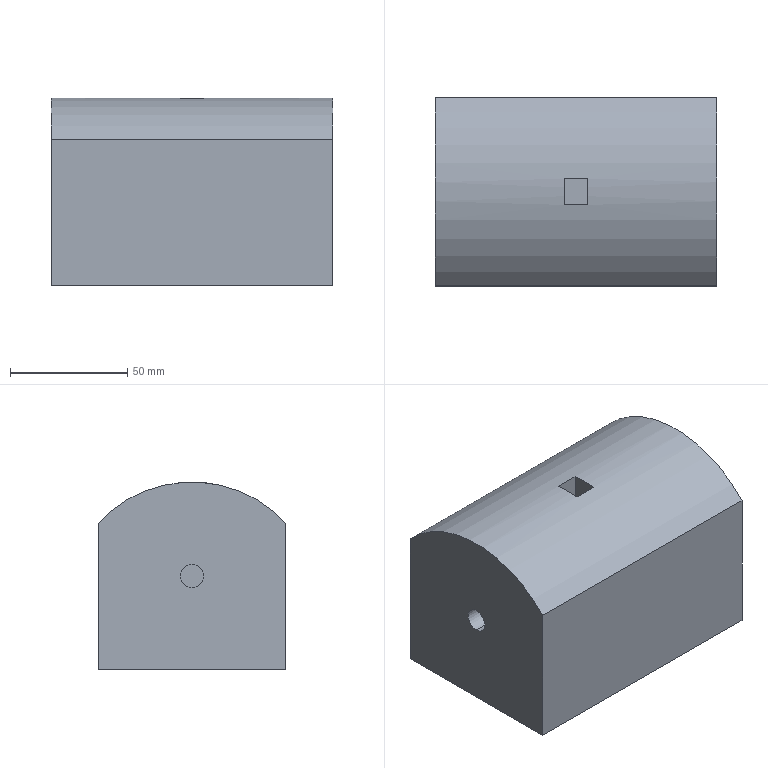Part | SolidWorks | features ICE 4, Extrusion 1 | 1 solid | 17 faces | box 120 x 80 x 80 mm | volume 704237 mm3 | plane 12 | cylinder 5 | commonest cylinder face diameters 10 x4 109 x1
STEP:
#1=CARTESIAN_POINT('',(60.,0.,35.));
#2=VERTEX_POINT('',#1);
#3=CARTESIAN_POINT('',(60.,0.,45.));
#4=VERTEX_POINT('',#3);
#5=CARTESIAN_POINT('',(60.,0.,40.));
#6=DIRECTION('',(-1.,0.,0.));
#7=DIRECTION('',(0.,0.,1.));
#8=AXIS2_PLACEMENT_3D('',#5,#6,#7);
#9=CIRCLE('',#8,5.);
#10=EDGE_CURVE('',#2,#4,#9,.T.);
#11=ORIENTED_EDGE('',*,*,#10,.F.);
#12=CARTESIAN_POINT('',(5.,0.,35.));
#13=VERTEX_POINT('',#12);
#14=CARTESIAN_POINT('',(60.,0.,35.));
#15=DIRECTION('',(-1.,0.,0.));
#16=VECTOR('',#15,1000.);
#17=LINE('',#14,#16);
#18=EDGE_CURVE('',#2,#13,#17,.T.);
#19=ORIENTED_EDGE('',*,*,#18,.T.);
#20=CARTESIAN_POINT('',(5.,0.,45.));
#21=VERTEX_POINT('',#20);
#22=CARTESIAN_POINT('',(5.,0.,40.));
#23=DIRECTION('',(1.,0.,0.));
#24=DIRECTION('',(0.,0.,-1.));
#25=AXIS2_PLACEMENT_3D('',#22,#23,#24);
#26=CIRCLE('',#25,5.);
#27=EDGE_CURVE('',#21,#13,#26,.T.);
#28=ORIENTED_EDGE('',*,*,#27,.F.);
#29=CARTESIAN_POINT('',(60.,0.,45.));
#30=DIRECTION('',(-1.,0.,0.));
#31=VECTOR('',#30,1000.);
#32=LINE('',#29,#31);
#33=EDGE_CURVE('',#4,#21,#32,.T.);
#34=ORIENTED_EDGE('',*,*,#33,.F.);
#35=EDGE_LOOP('',(#11,#19,#28,#34));
#36=FACE_OUTER_BOUND('',#35,.T.);
#37=CARTESIAN_POINT('',(60.,0.,40.));
#38=DIRECTION('',(-1.,0.,0.));
#39=DIRECTION('',(0.,0.,1.));
#40=AXIS2_PLACEMENT_3D('',#37,#38,#39);
#41=CYLINDRICAL_SURFACE('',#40,5.);
#42=ADVANCED_FACE('',(#36),#41,.F.);
#43=CARTESIAN_POINT('',(-5.,0.,35.));
#44=VERTEX_POINT('',#43);
#45=CARTESIAN_POINT('',(-5.,0.,45.));
#46=VERTEX_POINT('',#45);
#47=CARTESIAN_POINT('',(-5.,0.,40.));
#48=DIRECTION('',(-1.,0.,0.));
#49=DIRECTION('',(0.,0.,1.));
#50=AXIS2_PLACEMENT_3D('',#47,#48,#49);
#51=CIRCLE('',#50,5.);
#52=EDGE_CURVE('',#44,#46,#51,.T.);
#53=ORIENTED_EDGE('',*,*,#52,.F.);
#54=CARTESIAN_POINT('',(-60.,0.,35.));
#55=VERTEX_POINT('',#54);
#56=CARTESIAN_POINT('',(60.,0.,35.));
#57=DIRECTION('',(-1.,0.,0.));
#58=VECTOR('',#57,1000.);
#59=LINE('',#56,#58);
#60=EDGE_CURVE('',#44,#55,#59,.T.);
#61=ORIENTED_EDGE('',*,*,#60,.T.);
#62=CARTESIAN_POINT('',(-60.,0.,45.));
#63=VERTEX_POINT('',#62);
#64=CARTESIAN_POINT('',(-60.,0.,40.));
#65=DIRECTION('',(-1.,0.,0.));
#66=DIRECTION('',(0.,0.,1.));
#67=AXIS2_PLACEMENT_3D('',#64,#65,#66);
#68=CIRCLE('',#67,5.);
#69=EDGE_CURVE('',#55,#63,#68,.T.);
#70=ORIENTED_EDGE('',*,*,#69,.T.);
#71=CARTESIAN_POINT('',(60.,0.,45.));
#72=DIRECTION('',(-1.,0.,0.));
#73=VECTOR('',#72,1000.);
#74=LINE('',#71,#73);
#75=EDGE_CURVE('',#46,#63,#74,.T.);
#76=ORIENTED_EDGE('',*,*,#75,.F.);
#77=EDGE_LOOP('',(#53,#61,#70,#76));
#78=FACE_OUTER_BOUND('',#77,.T.);
#79=CARTESIAN_POINT('',(60.,0.,40.));
#80=DIRECTION('',(-1.,0.,0.));
#81=DIRECTION('',(0.,0.,1.));
#82=AXIS2_PLACEMENT_3D('',#79,#80,#81);
#83=CYLINDRICAL_SURFACE('',#82,5.);
#84=ADVANCED_FACE('',(#78),#83,.F.);
#85=ORIENTED_EDGE('',*,*,#60,.F.);
#86=CARTESIAN_POINT('',(-5.,0.,40.));
#87=DIRECTION('',(-1.,0.,0.));
#88=DIRECTION('',(0.,0.,1.));
#89=AXIS2_PLACEMENT_3D('',#86,#87,#88);
#90=CIRCLE('',#89,5.);
#91=EDGE_CURVE('',#46,#44,#90,.T.);
#92=ORIENTED_EDGE('',*,*,#91,.F.);
#93=ORIENTED_EDGE('',*,*,#75,.T.);
#94=CARTESIAN_POINT('',(-60.,0.,40.));
#95=DIRECTION('',(-1.,0.,0.));
#96=DIRECTION('',(0.,0.,1.));
#97=AXIS2_PLACEMENT_3D('',#94,#95,#96);
#98=CIRCLE('',#97,5.);
#99=EDGE_CURVE('',#63,#55,#98,.T.);
#100=ORIENTED_EDGE('',*,*,#99,.T.);
#101=EDGE_LOOP('',(#85,#92,#93,#100));
#102=FACE_OUTER_BOUND('',#101,.T.);
#103=CARTESIAN_POINT('',(60.,0.,40.));
#104=DIRECTION('',(-1.,0.,0.));
#105=DIRECTION('',(0.,0.,1.));
#106=AXIS2_PLACEMENT_3D('',#103,#104,#105);
#107=CYLINDRICAL_SURFACE('',#106,5.);
#108=ADVANCED_FACE('',(#102),#107,.F.);
#109=CARTESIAN_POINT('',(60.,0.,40.));
#110=DIRECTION('',(-1.,0.,0.));
#111=DIRECTION('',(0.,0.,1.));
#112=AXIS2_PLACEMENT_3D('',#109,#110,#111);
#113=CIRCLE('',#112,5.);
#114=EDGE_CURVE('',#4,#2,#113,.T.);
#115=ORIENTED_EDGE('',*,*,#114,.T.);
#116=ORIENTED_EDGE('',*,*,#10,.T.);
#117=EDGE_LOOP('',(#115,#116));
#118=FACE_BOUND('',#117,.T.);
#119=CARTESIAN_POINT('',(60.,40.,62.517));
#120=VERTEX_POINT('',#119);
#121=CARTESIAN_POINT('',(60.,-40.,62.517));
#122=VERTEX_POINT('',#121);
#123=CARTESIAN_POINT('',(60.,0.,25.5));
#124=DIRECTION('',(1.,0.,0.));
#125=DIRECTION('',(0.,0.,-1.));
#126=AXIS2_PLACEMENT_3D('',#123,#124,#125);
#127=CIRCLE('',#126,54.5);
#128=EDGE_CURVE('',#120,#122,#127,.T.);
#129=ORIENTED_EDGE('',*,*,#128,.T.);
#130=CARTESIAN_POINT('',(60.,-40.,0.));
#131=VERTEX_POINT('',#130);
#132=CARTESIAN_POINT('',(60.,-40.,80.));
#133=DIRECTION('',(0.,0.,-1.));
#134=VECTOR('',#133,1000.);
#135=LINE('',#132,#134);
#136=EDGE_CURVE('',#122,#131,#135,.T.);
#137=ORIENTED_EDGE('',*,*,#136,.T.);
#138=CARTESIAN_POINT('',(60.,40.,0.));
#139=VERTEX_POINT('',#138);
#140=CARTESIAN_POINT('',(60.,-40.,0.));
#141=DIRECTION('',(0.,1.,0.));
#142=VECTOR('',#141,1000.);
#143=LINE('',#140,#142);
#144=EDGE_CURVE('',#131,#139,#143,.T.);
#145=ORIENTED_EDGE('',*,*,#144,.T.);
#146=CARTESIAN_POINT('',(60.,40.,80.));
#147=DIRECTION('',(0.,0.,-1.));
#148=VECTOR('',#147,1000.);
#149=LINE('',#146,#148);
#150=EDGE_CURVE('',#120,#139,#149,.T.);
#151=ORIENTED_EDGE('',*,*,#150,.F.);
#152=EDGE_LOOP('',(#129,#137,#145,#151));
#153=FACE_OUTER_BOUND('',#152,.T.);
#154=CARTESIAN_POINT('',(60.,-40.,80.));
#155=DIRECTION('',(-1.,0.,0.));
#156=DIRECTION('',(0.,0.,1.));
#157=AXIS2_PLACEMENT_3D('',#154,#155,#156);
#158=PLANE('',#157);
#159=ADVANCED_FACE('',(#118,#153),#158,.F.);
#160=ORIENTED_EDGE('',*,*,#99,.F.);
#161=ORIENTED_EDGE('',*,*,#69,.F.);
#162=EDGE_LOOP('',(#160,#161));
#163=FACE_BOUND('',#162,.T.);
#164=CARTESIAN_POINT('',(-60.,-40.,62.517));
#165=VERTEX_POINT('',#164);
#166=CARTESIAN_POINT('',(-60.,-40.,0.));
#167=VERTEX_POINT('',#166);
#168=CARTESIAN_POINT('',(-60.,-40.,80.));
#169=DIRECTION('',(0.,0.,-1.));
#170=VECTOR('',#169,1000.);
#171=LINE('',#168,#170);
#172=EDGE_CURVE('',#165,#167,#171,.T.);
#173=ORIENTED_EDGE('',*,*,#172,.F.);
#174=CARTESIAN_POINT('',(-60.,40.,62.517));
#175=VERTEX_POINT('',#174);
#176=CARTESIAN_POINT('',(-60.,0.,25.5));
#177=DIRECTION('',(1.,0.,0.));
#178=DIRECTION('',(0.,0.,-1.));
#179=AXIS2_PLACEMENT_3D('',#176,#177,#178);
#180=CIRCLE('',#179,54.5);
#181=EDGE_CURVE('',#175,#165,#180,.T.);
#182=ORIENTED_EDGE('',*,*,#181,.F.);
#183=CARTESIAN_POINT('',(-60.,40.,0.));
#184=VERTEX_POINT('',#183);
#185=CARTESIAN_POINT('',(-60.,40.,80.));
#186=DIRECTION('',(0.,0.,-1.));
#187=VECTOR('',#186,1000.);
#188=LINE('',#185,#187);
#189=EDGE_CURVE('',#175,#184,#188,.T.);
#190=ORIENTED_EDGE('',*,*,#189,.T.);
#191=CARTESIAN_POINT('',(-60.,-40.,0.));
#192=DIRECTION('',(0.,-1.,0.));
#193=VECTOR('',#192,1000.);
#194=LINE('',#191,#193);
#195=EDGE_CURVE('',#184,#167,#194,.T.);
#196=ORIENTED_EDGE('',*,*,#195,.T.);
#197=EDGE_LOOP('',(#173,#182,#190,#196));
#198=FACE_OUTER_BOUND('',#197,.T.);
#199=CARTESIAN_POINT('',(-60.,-40.,80.));
#200=DIRECTION('',(1.,0.,0.));
#201=DIRECTION('',(0.,0.,-1.));
#202=AXIS2_PLACEMENT_3D('',#199,#200,#201);
#203=PLANE('',#202);
#204=ADVANCED_FACE('',(#163,#198),#203,.F.);
#205=CARTESIAN_POINT('',(-60.,-40.,62.517));
#206=DIRECTION('',(1.,0.,0.));
#207=VECTOR('',#206,1000.);
#208=LINE('',#205,#207);
#209=EDGE_CURVE('',#165,#122,#208,.T.);
#210=ORIENTED_EDGE('',*,*,#209,.F.);
#211=ORIENTED_EDGE('',*,*,#172,.T.);
#212=CARTESIAN_POINT('',(-60.,-40.,0.));
#213=DIRECTION('',(1.,0.,0.));
#214=VECTOR('',#213,1000.);
#215=LINE('',#212,#214);
#216=EDGE_CURVE('',#167,#131,#215,.T.);
#217=ORIENTED_EDGE('',*,*,#216,.T.);
#218=ORIENTED_EDGE('',*,*,#136,.F.);
#219=EDGE_LOOP('',(#210,#211,#217,#218));
#220=FACE_OUTER_BOUND('',#219,.T.);
#221=CARTESIAN_POINT('',(-60.,-40.,80.));
#222=DIRECTION('',(0.,1.,0.));
#223=DIRECTION('',(0.,0.,1.));
#224=AXIS2_PLACEMENT_3D('',#221,#222,#223);
#225=PLANE('',#224);
#226=ADVANCED_FACE('',(#220),#225,.F.);
#227=CARTESIAN_POINT('',(-60.,40.,62.517));
#228=DIRECTION('',(1.,0.,0.));
#229=VECTOR('',#228,1000.);
#230=LINE('',#227,#229);
#231=EDGE_CURVE('',#175,#120,#230,.T.);
#232=ORIENTED_EDGE('',*,*,#231,.T.);
#233=ORIENTED_EDGE('',*,*,#150,.T.);
#234=CARTESIAN_POINT('',(-60.,40.,0.));
#235=DIRECTION('',(-1.,0.,0.));
#236=VECTOR('',#235,1000.);
#237=LINE('',#234,#236);
#238=EDGE_CURVE('',#139,#184,#237,.T.);
#239=ORIENTED_EDGE('',*,*,#238,.T.);
#240=ORIENTED_EDGE('',*,*,#189,.F.);
#241=EDGE_LOOP('',(#232,#233,#239,#240));
#242=FACE_OUTER_BOUND('',#241,.T.);
#243=CARTESIAN_POINT('',(-60.,40.,80.));
#244=DIRECTION('',(0.,-1.,0.));
#245=DIRECTION('',(0.,0.,-1.));
#246=AXIS2_PLACEMENT_3D('',#243,#244,#245);
#247=PLANE('',#246);
#248=ADVANCED_FACE('',(#242),#247,.F.);
#249=ORIENTED_EDGE('',*,*,#144,.F.);
#250=ORIENTED_EDGE('',*,*,#216,.F.);
#251=ORIENTED_EDGE('',*,*,#195,.F.);
#252=ORIENTED_EDGE('',*,*,#238,.F.);
#253=EDGE_LOOP('',(#249,#250,#251,#252));
#254=FACE_OUTER_BOUND('',#253,.T.);
#255=CARTESIAN_POINT('',(0.,0.,0.));
#256=DIRECTION('',(0.,0.,-1.));
#257=DIRECTION('',(-1.,0.,0.));
#258=AXIS2_PLACEMENT_3D('',#255,#256,#257);
#259=PLANE('',#258);
#260=ADVANCED_FACE('',(#254),#259,.T.);
#261=ORIENTED_EDGE('',*,*,#18,.F.);
#262=ORIENTED_EDGE('',*,*,#114,.F.);
#263=ORIENTED_EDGE('',*,*,#33,.T.);
#264=CARTESIAN_POINT('',(5.,0.,40.));
#265=DIRECTION('',(1.,0.,0.));
#266=DIRECTION('',(0.,0.,-1.));
#267=AXIS2_PLACEMENT_3D('',#264,#265,#266);
#268=CIRCLE('',#267,5.);
#269=EDGE_CURVE('',#13,#21,#268,.T.);
#270=ORIENTED_EDGE('',*,*,#269,.F.);
#271=EDGE_LOOP('',(#261,#262,#263,#270));
#272=FACE_OUTER_BOUND('',#271,.T.);
#273=CARTESIAN_POINT('',(60.,0.,40.));
#274=DIRECTION('',(-1.,0.,0.));
#275=DIRECTION('',(0.,0.,1.));
#276=AXIS2_PLACEMENT_3D('',#273,#274,#275);
#277=CYLINDRICAL_SURFACE('',#276,5.);
#278=ADVANCED_FACE('',(#272),#277,.F.);
#279=CARTESIAN_POINT('',(5.,-5.59,79.713));
#280=VERTEX_POINT('',#279);
#281=CARTESIAN_POINT('',(-5.,-5.59,79.713));
#282=VERTEX_POINT('',#281);
#283=CARTESIAN_POINT('',(-60.,-5.59,79.713));
#284=DIRECTION('',(-1.,0.,0.));
#285=VECTOR('',#284,1000.);
#286=LINE('',#283,#285);
#287=EDGE_CURVE('',#280,#282,#286,.T.);
#288=ORIENTED_EDGE('',*,*,#287,.T.);
#289=CARTESIAN_POINT('',(-5.,5.59,79.713));
#290=VERTEX_POINT('',#289);
#291=CARTESIAN_POINT('',(-5.,0.,25.5));
#292=DIRECTION('',(-1.,0.,0.));
#293=DIRECTION('',(0.,0.,1.));
#294=AXIS2_PLACEMENT_3D('',#291,#292,#293);
#295=CIRCLE('',#294,54.5);
#296=EDGE_CURVE('',#282,#290,#295,.T.);
#297=ORIENTED_EDGE('',*,*,#296,.T.);
#298=CARTESIAN_POINT('',(5.,5.59,79.713));
#299=VERTEX_POINT('',#298);
#300=CARTESIAN_POINT('',(-60.,5.59,79.713));
#301=DIRECTION('',(1.,0.,0.));
#302=VECTOR('',#301,1000.);
#303=LINE('',#300,#302);
#304=EDGE_CURVE('',#290,#299,#303,.T.);
#305=ORIENTED_EDGE('',*,*,#304,.T.);
#306=CARTESIAN_POINT('',(5.,0.,25.5));
#307=DIRECTION('',(1.,0.,0.));
#308=DIRECTION('',(0.,0.,-1.));
#309=AXIS2_PLACEMENT_3D('',#306,#307,#308);
#310=CIRCLE('',#309,54.5);
#311=EDGE_CURVE('',#299,#280,#310,.T.);
#312=ORIENTED_EDGE('',*,*,#311,.T.);
#313=EDGE_LOOP('',(#288,#297,#305,#312));
#314=FACE_BOUND('',#313,.T.);
#315=ORIENTED_EDGE('',*,*,#128,.F.);
#316=ORIENTED_EDGE('',*,*,#231,.F.);
#317=ORIENTED_EDGE('',*,*,#181,.T.);
#318=ORIENTED_EDGE('',*,*,#209,.T.);
#319=EDGE_LOOP('',(#315,#316,#317,#318));
#320=FACE_OUTER_BOUND('',#319,.T.);
#321=CARTESIAN_POINT('',(-60.,0.,25.5));
#322=DIRECTION('',(1.,0.,0.));
#323=DIRECTION('',(0.,0.,-1.));
#324=AXIS2_PLACEMENT_3D('',#321,#322,#323);
#325=CYLINDRICAL_SURFACE('',#324,54.5);
#326=ADVANCED_FACE('',(#314,#320),#325,.T.);
#327=CARTESIAN_POINT('',(-5.,-5.59,50.));
#328=VERTEX_POINT('',#327);
#329=CARTESIAN_POINT('',(-5.,-5.59,80.001));
#330=DIRECTION('',(0.,0.,-1.));
#331=VECTOR('',#330,1000.);
#332=LINE('',#329,#331);
#333=EDGE_CURVE('',#282,#328,#332,.T.);
#334=ORIENTED_EDGE('',*,*,#333,.T.);
#335=CARTESIAN_POINT('',(-5.,5.59,50.));
#336=VERTEX_POINT('',#335);
#337=CARTESIAN_POINT('',(-5.,-5.59,50.));
#338=DIRECTION('',(0.,1.,0.));
#339=VECTOR('',#338,1000.);
#340=LINE('',#337,#339);
#341=EDGE_CURVE('',#328,#336,#340,.T.);
#342=ORIENTED_EDGE('',*,*,#341,.T.);
#343=CARTESIAN_POINT('',(-5.,5.59,80.001));
#344=DIRECTION('',(0.,0.,-1.));
#345=VECTOR('',#344,1000.);
#346=LINE('',#343,#345);
#347=EDGE_CURVE('',#290,#336,#346,.T.);
#348=ORIENTED_EDGE('',*,*,#347,.F.);
#349=ORIENTED_EDGE('',*,*,#296,.F.);
#350=EDGE_LOOP('',(#334,#342,#348,#349));
#351=FACE_OUTER_BOUND('',#350,.T.);
#352=CARTESIAN_POINT('',(-5.,-5.59,80.001));
#353=DIRECTION('',(-1.,0.,0.));
#354=DIRECTION('',(0.,0.,1.));
#355=AXIS2_PLACEMENT_3D('',#352,#353,#354);
#356=PLANE('',#355);
#357=ADVANCED_FACE('',(#351),#356,.F.);
#358=CARTESIAN_POINT('',(5.,5.59,50.));
#359=VERTEX_POINT('',#358);
#360=CARTESIAN_POINT('',(5.,5.59,80.001));
#361=DIRECTION('',(0.,0.,-1.));
#362=VECTOR('',#361,1000.);
#363=LINE('',#360,#362);
#364=EDGE_CURVE('',#299,#359,#363,.T.);
#365=ORIENTED_EDGE('',*,*,#364,.T.);
#366=CARTESIAN_POINT('',(5.,-5.59,50.));
#367=VERTEX_POINT('',#366);
#368=CARTESIAN_POINT('',(5.,-5.59,50.));
#369=DIRECTION('',(0.,-1.,0.));
#370=VECTOR('',#369,1000.);
#371=LINE('',#368,#370);
#372=EDGE_CURVE('',#359,#367,#371,.T.);
#373=ORIENTED_EDGE('',*,*,#372,.T.);
#374=CARTESIAN_POINT('',(5.,-5.59,80.001));
#375=DIRECTION('',(0.,0.,-1.));
#376=VECTOR('',#375,1000.);
#377=LINE('',#374,#376);
#378=EDGE_CURVE('',#280,#367,#377,.T.);
#379=ORIENTED_EDGE('',*,*,#378,.F.);
#380=ORIENTED_EDGE('',*,*,#311,.F.);
#381=EDGE_LOOP('',(#365,#373,#379,#380));
#382=FACE_OUTER_BOUND('',#381,.T.);
#383=CARTESIAN_POINT('',(5.,-5.59,80.001));
#384=DIRECTION('',(1.,0.,0.));
#385=DIRECTION('',(0.,0.,-1.));
#386=AXIS2_PLACEMENT_3D('',#383,#384,#385);
#387=PLANE('',#386);
#388=ADVANCED_FACE('',(#382),#387,.F.);
#389=ORIENTED_EDGE('',*,*,#378,.T.);
#390=CARTESIAN_POINT('',(5.,-5.59,50.));
#391=DIRECTION('',(-1.,0.,0.));
#392=VECTOR('',#391,1000.);
#393=LINE('',#390,#392);
#394=EDGE_CURVE('',#367,#328,#393,.T.);
#395=ORIENTED_EDGE('',*,*,#394,.T.);
#396=ORIENTED_EDGE('',*,*,#333,.F.);
#397=ORIENTED_EDGE('',*,*,#287,.F.);
#398=EDGE_LOOP('',(#389,#395,#396,#397));
#399=FACE_OUTER_BOUND('',#398,.T.);
#400=CARTESIAN_POINT('',(5.,-5.59,80.001));
#401=DIRECTION('',(0.,-1.,0.));
#402=DIRECTION('',(0.,0.,-1.));
#403=AXIS2_PLACEMENT_3D('',#400,#401,#402);
#404=PLANE('',#403);
#405=ADVANCED_FACE('',(#399),#404,.F.);
#406=ORIENTED_EDGE('',*,*,#347,.T.);
#407=CARTESIAN_POINT('',(5.,5.59,50.));
#408=DIRECTION('',(1.,0.,0.));
#409=VECTOR('',#408,1000.);
#410=LINE('',#407,#409);
#411=EDGE_CURVE('',#336,#359,#410,.T.);
#412=ORIENTED_EDGE('',*,*,#411,.T.);
#413=ORIENTED_EDGE('',*,*,#364,.F.);
#414=ORIENTED_EDGE('',*,*,#304,.F.);
#415=EDGE_LOOP('',(#406,#412,#413,#414));
#416=FACE_OUTER_BOUND('',#415,.T.);
#417=CARTESIAN_POINT('',(5.,5.59,80.001));
#418=DIRECTION('',(0.,1.,0.));
#419=DIRECTION('',(0.,0.,1.));
#420=AXIS2_PLACEMENT_3D('',#417,#418,#419);
#421=PLANE('',#420);
#422=ADVANCED_FACE('',(#416),#421,.F.);
#423=ORIENTED_EDGE('',*,*,#341,.F.);
#424=ORIENTED_EDGE('',*,*,#394,.F.);
#425=ORIENTED_EDGE('',*,*,#372,.F.);
#426=ORIENTED_EDGE('',*,*,#411,.F.);
#427=EDGE_LOOP('',(#423,#424,#425,#426));
#428=FACE_OUTER_BOUND('',#427,.T.);
#429=CARTESIAN_POINT('',(0.,0.,50.));
#430=DIRECTION('',(0.,0.,1.));
#431=DIRECTION('',(1.,0.,0.));
#432=AXIS2_PLACEMENT_3D('',#429,#430,#431);
#433=PLANE('',#432);
#434=ADVANCED_FACE('',(#428),#433,.T.);
#435=ORIENTED_EDGE('',*,*,#27,.T.);
#436=ORIENTED_EDGE('',*,*,#269,.T.);
#437=EDGE_LOOP('',(#435,#436));
#438=FACE_OUTER_BOUND('',#437,.T.);
#439=CARTESIAN_POINT('',(5.,-5.59,50.));
#440=DIRECTION('',(1.,0.,0.));
#441=DIRECTION('',(0.,0.,-1.));
#442=AXIS2_PLACEMENT_3D('',#439,#440,#441);
#443=PLANE('',#442);
#444=ADVANCED_FACE('',(#438),#443,.T.);
#445=ORIENTED_EDGE('',*,*,#91,.T.);
#446=ORIENTED_EDGE('',*,*,#52,.T.);
#447=EDGE_LOOP('',(#445,#446));
#448=FACE_OUTER_BOUND('',#447,.T.);
#449=CARTESIAN_POINT('',(-5.,-5.59,50.));
#450=DIRECTION('',(-1.,0.,0.));
#451=DIRECTION('',(0.,0.,1.));
#452=AXIS2_PLACEMENT_3D('',#449,#450,#451);
#453=PLANE('',#452);
#454=ADVANCED_FACE('',(#448),#453,.T.);
#455=CLOSED_SHELL('',(#42,#84,#108,#159,#204,#226,#248,#260,#278,#326,#357,#388,#405,#422,#434,#444,#454));
#456=MANIFOLD_SOLID_BREP('',#455);
#457=CARTESIAN_POINT('',(0.,0.,0.));
#458=DIRECTION('',(0.,0.,1.));
#459=DIRECTION('',(1.,0.,0.));
#460=AXIS2_PLACEMENT_3D('',#457,#458,#459);
#461=(LENGTH_UNIT()NAMED_UNIT(*)SI_UNIT(.MILLI.,.METRE.));
#462=UNCERTAINTY_MEASURE_WITH_UNIT(LENGTH_MEASURE(0.00001),#461,'','');
#463=(NAMED_UNIT(*)PLANE_ANGLE_UNIT()SI_UNIT($,.RADIAN.));
#464=(NAMED_UNIT(*)SI_UNIT($,.STERADIAN.)SOLID_ANGLE_UNIT());
#465=(GEOMETRIC_REPRESENTATION_CONTEXT(3)GLOBAL_UNCERTAINTY_ASSIGNED_CONTEXT((#462))GLOBAL_UNIT_ASSIGNED_CONTEXT((#461,#463,#464))REPRESENTATION_CONTEXT('',''));
#466=ADVANCED_BREP_SHAPE_REPRESENTATION('',(#456,#460),#465);